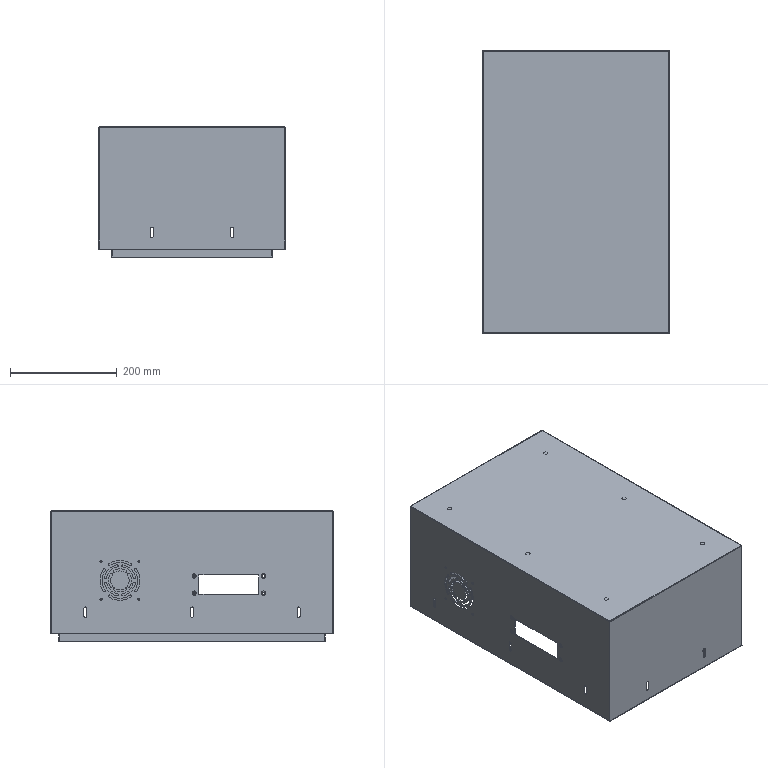Part | STEP file | Electrical Cabinet Base | 1 solid | 454 faces | box 350 x 530 x 243.8 mm | volume 759482 mm3 | cylinder 266 | plane 164 | cone 12 | spline 12 | commonest cylinder face diameters 4 x88 5 x34 3.3 x20 8 x20 4.2 x16 0.02 x12